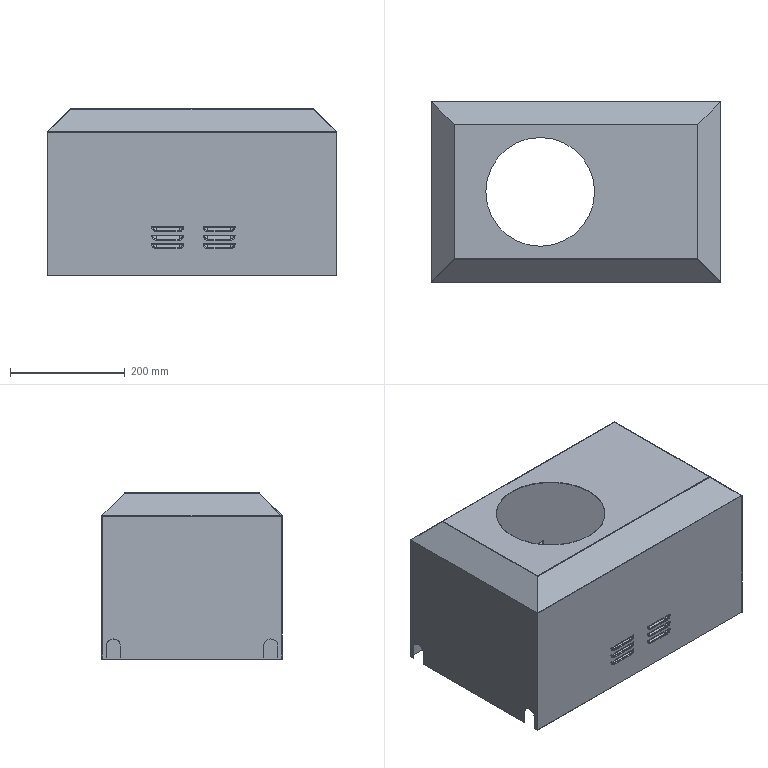Part | STEP file | 101000007773 | 2 solids | 255 faces | box 505 x 315 x 290 mm | volume 663603 mm3 | torus 72 | plane 61 | cylinder 60 | sphere 60 | spline 2 | commonest cylinder face diameters 2 x13 4 x13 12 x12 14 x12 25 x6 190 x4